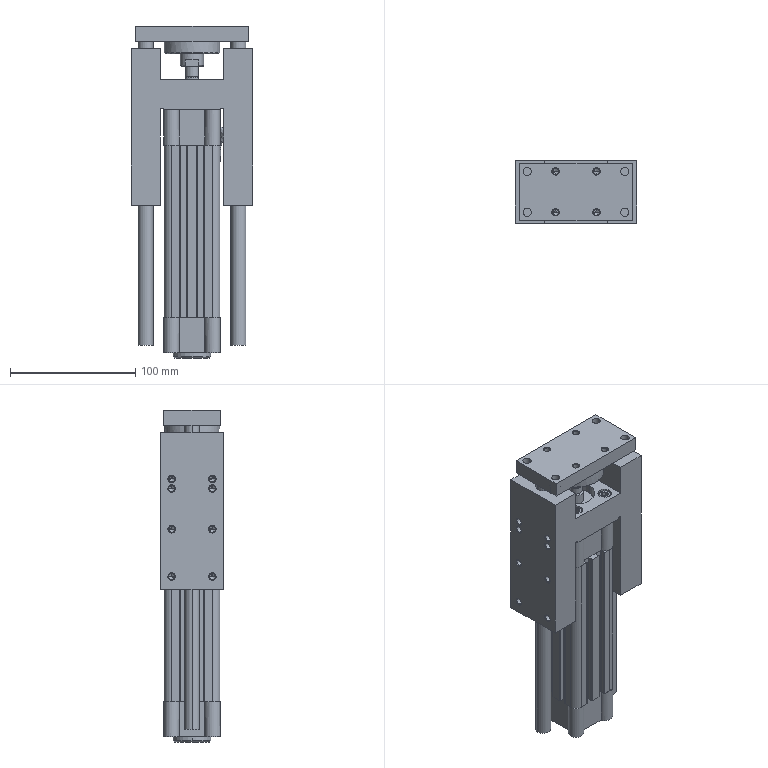Part | STEP file | 535411 DNCI-32-100-P-A-FENG-MS---(asm_0_)(control position cylinder 100)_5 | 8 solids | 676 faces | box 97 x 50 x 265 mm | volume 701103 mm3 | cylinder 230 | cone 227 | plane 215 | spline 4 | commonest cylinder face diameters 4.917 x56 0.6 x24 0.8 x24 6 x24 6.6 x16 11 x16